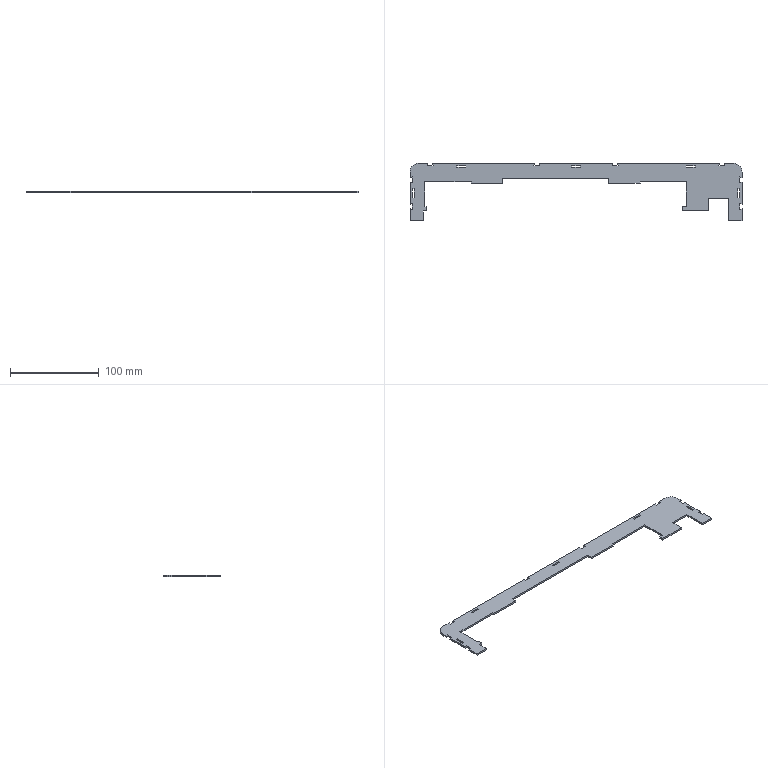Part | STEP file | xzz-004-1 | 1 solid | 82 faces | box 373.4 x 64.7 x 2 mm | volume 19566 mm3 | plane 80 | cylinder 2 | commonest cylinder face diameters 20 x2